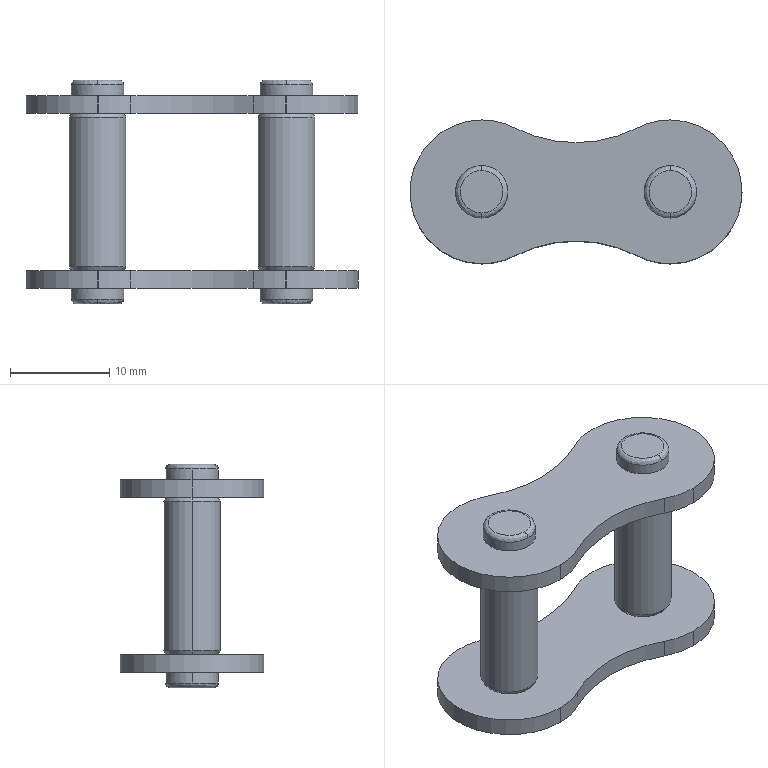Part | STEP file | 12b-1_01 | 1 solid | 62 faces | box 33.5 x 14.5 x 22.6 mm | volume 2362 mm3 | cylinder 30 | plane 16 | spline 8 | cone 8 | commonest cylinder face diameters 14.5 x14 5.29 x8 5.725 x4 27.08 x4